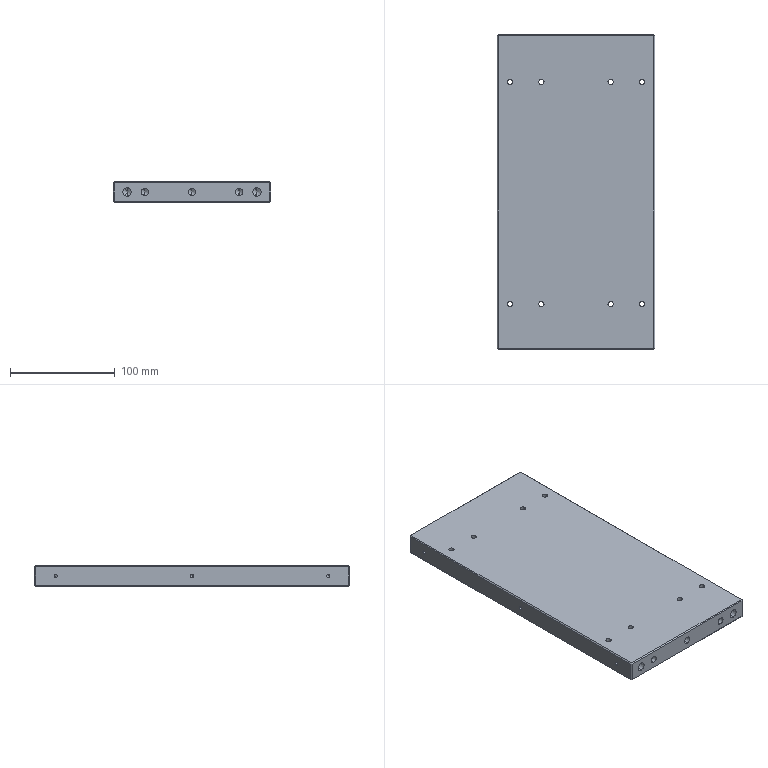Part | SolidWorks | features HoleWzd 5, MirrorPattern 2, Chamfer 1, Extrusion 1 | 1 solid | 106 faces | box 150 x 300 x 20 mm | volume 887361 mm3 | cylinder 48 | cone 32 | plane 26 | commonest cylinder face diameters 5 x16 3.3 x12 6.8 x12 8 x8